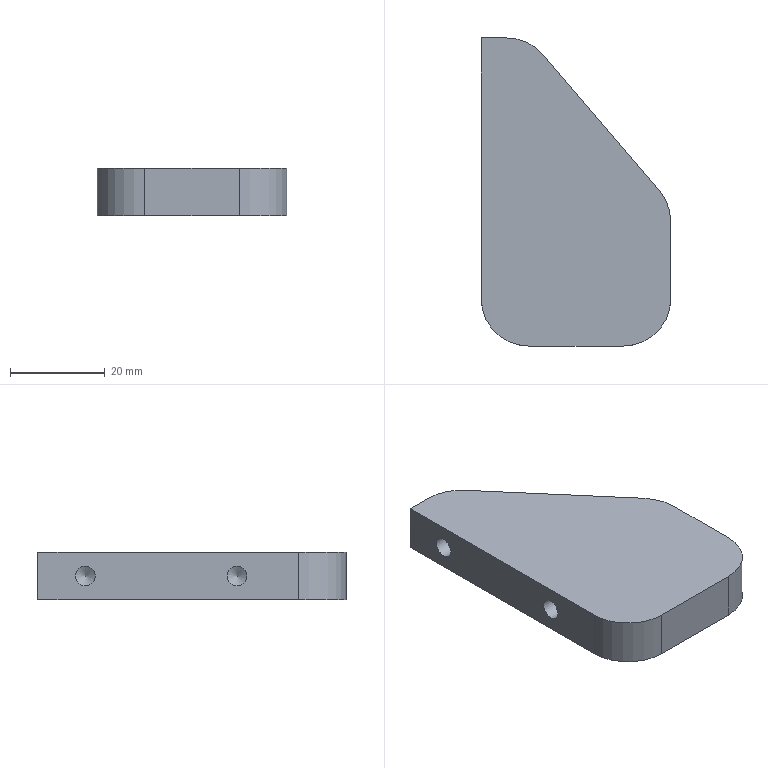Part | NX | 1 solid | 15 faces | box 40 x 65 x 10 mm | volume 19921 mm3 | plane 7 | cylinder 6 | cone 2 | commonest cylinder face diameters 20 x4 4.2 x2
STEP:
#1=CARTESIAN_POINT('',(-20.,22.5,2.1));
#2=VERTEX_POINT('',#1);
#3=CARTESIAN_POINT('',(-20.,22.5,0.));
#4=DIRECTION('',(-1.,0.,0.));
#5=DIRECTION('',(0.,0.,1.));
#6=AXIS2_PLACEMENT_3D('',#3,#4,#5);
#7=CIRCLE('',#6,2.1);
#8=EDGE_CURVE('',#2,#2,#7,.T.);
#9=ORIENTED_EDGE('',*,*,#8,.F.);
#10=EDGE_LOOP('',(#9));
#11=FACE_BOUND('',#10,.T.);
#12=CARTESIAN_POINT('',(-20.,-9.5,2.1));
#13=VERTEX_POINT('',#12);
#14=CARTESIAN_POINT('',(-20.,-9.5,0.));
#15=DIRECTION('',(-1.,0.,0.));
#16=DIRECTION('',(0.,0.,1.));
#17=AXIS2_PLACEMENT_3D('',#14,#15,#16);
#18=CIRCLE('',#17,2.1);
#19=EDGE_CURVE('',#13,#13,#18,.T.);
#20=ORIENTED_EDGE('',*,*,#19,.F.);
#21=EDGE_LOOP('',(#20));
#22=FACE_BOUND('',#21,.T.);
#23=CARTESIAN_POINT('',(-20.,32.5,-5.));
#24=VERTEX_POINT('',#23);
#25=CARTESIAN_POINT('',(-20.,-22.5,-5.));
#26=VERTEX_POINT('',#25);
#27=CARTESIAN_POINT('',(-20.,32.5,-5.));
#28=DIRECTION('',(0.,-1.,0.));
#29=VECTOR('',#28,1000.);
#30=LINE('',#27,#29);
#31=EDGE_CURVE('',#24,#26,#30,.T.);
#32=ORIENTED_EDGE('',*,*,#31,.T.);
#33=CARTESIAN_POINT('',(-20.,-22.5,5.));
#34=VERTEX_POINT('',#33);
#35=CARTESIAN_POINT('',(-20.,-22.5,5.));
#36=DIRECTION('',(0.,0.,-1.));
#37=VECTOR('',#36,1000.);
#38=LINE('',#35,#37);
#39=EDGE_CURVE('',#26,#34,#38,.F.);
#40=ORIENTED_EDGE('',*,*,#39,.T.);
#41=CARTESIAN_POINT('',(-20.,32.5,5.));
#42=VERTEX_POINT('',#41);
#43=CARTESIAN_POINT('',(-20.,32.5,5.));
#44=DIRECTION('',(0.,-1.,0.));
#45=VECTOR('',#44,1000.);
#46=LINE('',#43,#45);
#47=EDGE_CURVE('',#42,#34,#46,.T.);
#48=ORIENTED_EDGE('',*,*,#47,.F.);
#49=CARTESIAN_POINT('',(-20.,32.5,5.));
#50=DIRECTION('',(0.,0.,-1.));
#51=VECTOR('',#50,1000.);
#52=LINE('',#49,#51);
#53=EDGE_CURVE('',#42,#24,#52,.T.);
#54=ORIENTED_EDGE('',*,*,#53,.T.);
#55=EDGE_LOOP('',(#32,#40,#48,#54));
#56=FACE_BOUND('',#55,.T.);
#57=CARTESIAN_POINT('',(-20.,32.5,5.));
#58=DIRECTION('',(1.,0.,0.));
#59=DIRECTION('',(0.,1.,0.));
#60=AXIS2_PLACEMENT_3D('',#57,#58,#59);
#61=PLANE('',#60);
#62=ADVANCED_FACE('',(#11,#22,#56),#61,.F.);
#63=CARTESIAN_POINT('',(-10.,-32.5,5.));
#64=VERTEX_POINT('',#63);
#65=CARTESIAN_POINT('',(10.,-32.5,5.));
#66=VERTEX_POINT('',#65);
#67=CARTESIAN_POINT('',(20.,-32.5,5.));
#68=DIRECTION('',(1.,0.,0.));
#69=VECTOR('',#68,1000.);
#70=LINE('',#67,#69);
#71=EDGE_CURVE('',#64,#66,#70,.T.);
#72=ORIENTED_EDGE('',*,*,#71,.F.);
#73=CARTESIAN_POINT('',(-10.,-32.5,-5.));
#74=VERTEX_POINT('',#73);
#75=CARTESIAN_POINT('',(-10.,-32.5,5.));
#76=DIRECTION('',(0.,0.,-1.));
#77=VECTOR('',#76,1000.);
#78=LINE('',#75,#77);
#79=EDGE_CURVE('',#64,#74,#78,.T.);
#80=ORIENTED_EDGE('',*,*,#79,.T.);
#81=CARTESIAN_POINT('',(10.,-32.5,-5.));
#82=VERTEX_POINT('',#81);
#83=CARTESIAN_POINT('',(20.,-32.5,-5.));
#84=DIRECTION('',(1.,0.,0.));
#85=VECTOR('',#84,1000.);
#86=LINE('',#83,#85);
#87=EDGE_CURVE('',#74,#82,#86,.T.);
#88=ORIENTED_EDGE('',*,*,#87,.T.);
#89=CARTESIAN_POINT('',(10.,-32.5,5.));
#90=DIRECTION('',(0.,0.,-1.));
#91=VECTOR('',#90,1000.);
#92=LINE('',#89,#91);
#93=EDGE_CURVE('',#82,#66,#92,.F.);
#94=ORIENTED_EDGE('',*,*,#93,.T.);
#95=EDGE_LOOP('',(#72,#80,#88,#94));
#96=FACE_BOUND('',#95,.T.);
#97=CARTESIAN_POINT('',(20.,-32.5,5.));
#98=DIRECTION('',(0.,1.,0.));
#99=DIRECTION('',(0.,0.,1.));
#100=AXIS2_PLACEMENT_3D('',#97,#98,#99);
#101=PLANE('',#100);
#102=ADVANCED_FACE('',(#96),#101,.F.);
#103=CARTESIAN_POINT('',(20.,-22.5,-5.));
#104=VERTEX_POINT('',#103);
#105=CARTESIAN_POINT('',(20.,-6.199,-5.));
#106=VERTEX_POINT('',#105);
#107=CARTESIAN_POINT('',(20.,32.5,-5.));
#108=DIRECTION('',(0.,1.,0.));
#109=VECTOR('',#108,1000.);
#110=LINE('',#107,#109);
#111=EDGE_CURVE('',#104,#106,#110,.T.);
#112=ORIENTED_EDGE('',*,*,#111,.T.);
#113=CARTESIAN_POINT('',(20.,-6.199,5.));
#114=VERTEX_POINT('',#113);
#115=CARTESIAN_POINT('',(20.,-6.199,5.));
#116=DIRECTION('',(0.,0.,-1.));
#117=VECTOR('',#116,1000.);
#118=LINE('',#115,#117);
#119=EDGE_CURVE('',#106,#114,#118,.F.);
#120=ORIENTED_EDGE('',*,*,#119,.T.);
#121=CARTESIAN_POINT('',(20.,-22.5,5.));
#122=VERTEX_POINT('',#121);
#123=CARTESIAN_POINT('',(20.,32.5,5.));
#124=DIRECTION('',(0.,1.,0.));
#125=VECTOR('',#124,1000.);
#126=LINE('',#123,#125);
#127=EDGE_CURVE('',#122,#114,#126,.T.);
#128=ORIENTED_EDGE('',*,*,#127,.F.);
#129=CARTESIAN_POINT('',(20.,-22.5,5.));
#130=DIRECTION('',(0.,0.,-1.));
#131=VECTOR('',#130,1000.);
#132=LINE('',#129,#131);
#133=EDGE_CURVE('',#122,#104,#132,.T.);
#134=ORIENTED_EDGE('',*,*,#133,.T.);
#135=EDGE_LOOP('',(#112,#120,#128,#134));
#136=FACE_BOUND('',#135,.T.);
#137=CARTESIAN_POINT('',(20.,32.5,5.));
#138=DIRECTION('',(-1.,0.,0.));
#139=DIRECTION('',(0.,-1.,0.));
#140=AXIS2_PLACEMENT_3D('',#137,#138,#139);
#141=PLANE('',#140);
#142=ADVANCED_FACE('',(#136),#141,.F.);
#143=CARTESIAN_POINT('',(-14.599,32.5,5.));
#144=VERTEX_POINT('',#143);
#145=CARTESIAN_POINT('',(20.,32.5,5.));
#146=DIRECTION('',(-1.,0.,0.));
#147=VECTOR('',#146,1000.);
#148=LINE('',#145,#147);
#149=EDGE_CURVE('',#144,#42,#148,.T.);
#150=ORIENTED_EDGE('',*,*,#149,.F.);
#151=CARTESIAN_POINT('',(-14.599,32.5,-5.));
#152=VERTEX_POINT('',#151);
#153=CARTESIAN_POINT('',(-14.599,32.5,-5.));
#154=DIRECTION('',(0.,0.,1.));
#155=VECTOR('',#154,1000.);
#156=LINE('',#153,#155);
#157=EDGE_CURVE('',#144,#152,#156,.F.);
#158=ORIENTED_EDGE('',*,*,#157,.T.);
#159=CARTESIAN_POINT('',(20.,32.5,-5.));
#160=DIRECTION('',(-1.,0.,0.));
#161=VECTOR('',#160,1000.);
#162=LINE('',#159,#161);
#163=EDGE_CURVE('',#152,#24,#162,.T.);
#164=ORIENTED_EDGE('',*,*,#163,.T.);
#165=ORIENTED_EDGE('',*,*,#53,.F.);
#166=EDGE_LOOP('',(#150,#158,#164,#165));
#167=FACE_BOUND('',#166,.T.);
#168=CARTESIAN_POINT('',(20.,32.5,5.));
#169=DIRECTION('',(0.,-1.,0.));
#170=DIRECTION('',(1.,0.,0.));
#171=AXIS2_PLACEMENT_3D('',#168,#169,#170);
#172=PLANE('',#171);
#173=ADVANCED_FACE('',(#167),#172,.F.);
#174=ORIENTED_EDGE('',*,*,#127,.T.);
#175=CARTESIAN_POINT('',(17.593,0.3087,5.));
#176=VERTEX_POINT('',#175);
#177=CARTESIAN_POINT('',(10.,-6.199,5.));
#178=DIRECTION('',(0.,0.,-1.));
#179=DIRECTION('',(-1.,0.,0.));
#180=AXIS2_PLACEMENT_3D('',#177,#178,#179);
#181=CIRCLE('',#180,10.);
#182=EDGE_CURVE('',#114,#176,#181,.F.);
#183=ORIENTED_EDGE('',*,*,#182,.T.);
#184=CARTESIAN_POINT('',(-7.007,29.008,5.));
#185=VERTEX_POINT('',#184);
#186=CARTESIAN_POINT('',(-10.,32.5,5.));
#187=DIRECTION('',(0.6508,-0.7593,0.));
#188=VECTOR('',#187,1000.);
#189=LINE('',#186,#188);
#190=EDGE_CURVE('',#176,#185,#189,.F.);
#191=ORIENTED_EDGE('',*,*,#190,.T.);
#192=CARTESIAN_POINT('',(-14.599,22.5,5.));
#193=DIRECTION('',(0.,0.,-1.));
#194=DIRECTION('',(-1.,0.,0.));
#195=AXIS2_PLACEMENT_3D('',#192,#193,#194);
#196=CIRCLE('',#195,10.);
#197=EDGE_CURVE('',#185,#144,#196,.F.);
#198=ORIENTED_EDGE('',*,*,#197,.T.);
#199=ORIENTED_EDGE('',*,*,#149,.T.);
#200=ORIENTED_EDGE('',*,*,#47,.T.);
#201=CARTESIAN_POINT('',(-10.,-22.5,5.));
#202=DIRECTION('',(0.,0.,-1.));
#203=DIRECTION('',(-1.,0.,0.));
#204=AXIS2_PLACEMENT_3D('',#201,#202,#203);
#205=CIRCLE('',#204,10.);
#206=EDGE_CURVE('',#34,#64,#205,.F.);
#207=ORIENTED_EDGE('',*,*,#206,.T.);
#208=ORIENTED_EDGE('',*,*,#71,.T.);
#209=CARTESIAN_POINT('',(10.,-22.5,5.));
#210=DIRECTION('',(0.,0.,-1.));
#211=DIRECTION('',(-1.,0.,0.));
#212=AXIS2_PLACEMENT_3D('',#209,#210,#211);
#213=CIRCLE('',#212,10.);
#214=EDGE_CURVE('',#66,#122,#213,.F.);
#215=ORIENTED_EDGE('',*,*,#214,.T.);
#216=EDGE_LOOP('',(#174,#183,#191,#198,#199,#200,#207,#208,#215));
#217=FACE_BOUND('',#216,.T.);
#218=CARTESIAN_POINT('',(0.,0.,5.));
#219=DIRECTION('',(0.,0.,-1.));
#220=DIRECTION('',(-1.,0.,0.));
#221=AXIS2_PLACEMENT_3D('',#218,#219,#220);
#222=PLANE('',#221);
#223=ADVANCED_FACE('',(#217),#222,.F.);
#224=CARTESIAN_POINT('',(-7.007,29.008,-5.));
#225=VERTEX_POINT('',#224);
#226=CARTESIAN_POINT('',(17.593,0.3087,-5.));
#227=VERTEX_POINT('',#226);
#228=CARTESIAN_POINT('',(10.294,8.824,-5.));
#229=DIRECTION('',(-0.6508,0.7593,0.));
#230=VECTOR('',#229,1000.);
#231=LINE('',#228,#230);
#232=EDGE_CURVE('',#225,#227,#231,.F.);
#233=ORIENTED_EDGE('',*,*,#232,.T.);
#234=CARTESIAN_POINT('',(10.,-6.199,-5.));
#235=DIRECTION('',(0.,0.,-1.));
#236=DIRECTION('',(-1.,0.,0.));
#237=AXIS2_PLACEMENT_3D('',#234,#235,#236);
#238=CIRCLE('',#237,10.);
#239=EDGE_CURVE('',#227,#106,#238,.T.);
#240=ORIENTED_EDGE('',*,*,#239,.T.);
#241=ORIENTED_EDGE('',*,*,#111,.F.);
#242=CARTESIAN_POINT('',(10.,-22.5,-5.));
#243=DIRECTION('',(0.,0.,-1.));
#244=DIRECTION('',(-1.,0.,0.));
#245=AXIS2_PLACEMENT_3D('',#242,#243,#244);
#246=CIRCLE('',#245,10.);
#247=EDGE_CURVE('',#104,#82,#246,.T.);
#248=ORIENTED_EDGE('',*,*,#247,.T.);
#249=ORIENTED_EDGE('',*,*,#87,.F.);
#250=CARTESIAN_POINT('',(-10.,-22.5,-5.));
#251=DIRECTION('',(0.,0.,-1.));
#252=DIRECTION('',(-1.,0.,0.));
#253=AXIS2_PLACEMENT_3D('',#250,#251,#252);
#254=CIRCLE('',#253,10.);
#255=EDGE_CURVE('',#74,#26,#254,.T.);
#256=ORIENTED_EDGE('',*,*,#255,.T.);
#257=ORIENTED_EDGE('',*,*,#31,.F.);
#258=ORIENTED_EDGE('',*,*,#163,.F.);
#259=CARTESIAN_POINT('',(-14.599,22.5,-5.));
#260=DIRECTION('',(0.,0.,-1.));
#261=DIRECTION('',(-1.,0.,0.));
#262=AXIS2_PLACEMENT_3D('',#259,#260,#261);
#263=CIRCLE('',#262,10.);
#264=EDGE_CURVE('',#152,#225,#263,.T.);
#265=ORIENTED_EDGE('',*,*,#264,.T.);
#266=EDGE_LOOP('',(#233,#240,#241,#248,#249,#256,#257,#258,#265));
#267=FACE_BOUND('',#266,.T.);
#268=CARTESIAN_POINT('',(0.,0.,-5.));
#269=DIRECTION('',(0.,0.,-1.));
#270=DIRECTION('',(-1.,0.,0.));
#271=AXIS2_PLACEMENT_3D('',#268,#269,#270);
#272=PLANE('',#271);
#273=ADVANCED_FACE('',(#267),#272,.T.);
#274=ORIENTED_EDGE('',*,*,#190,.F.);
#275=CARTESIAN_POINT('',(17.593,0.3087,-5.));
#276=DIRECTION('',(0.,0.,1.));
#277=VECTOR('',#276,1000.);
#278=LINE('',#275,#277);
#279=EDGE_CURVE('',#176,#227,#278,.F.);
#280=ORIENTED_EDGE('',*,*,#279,.T.);
#281=ORIENTED_EDGE('',*,*,#232,.F.);
#282=CARTESIAN_POINT('',(-7.007,29.008,5.));
#283=DIRECTION('',(0.,0.,-1.));
#284=VECTOR('',#283,1000.);
#285=LINE('',#282,#284);
#286=EDGE_CURVE('',#225,#185,#285,.F.);
#287=ORIENTED_EDGE('',*,*,#286,.T.);
#288=EDGE_LOOP('',(#274,#280,#281,#287));
#289=FACE_BOUND('',#288,.T.);
#290=CARTESIAN_POINT('',(-10.,32.5,5.));
#291=DIRECTION('',(-0.7593,-0.6508,0.));
#292=DIRECTION('',(0.,0.,-1.));
#293=AXIS2_PLACEMENT_3D('',#290,#291,#292);
#294=PLANE('',#293);
#295=ADVANCED_FACE('',(#289),#294,.F.);
#296=CARTESIAN_POINT('',(-6.338,-9.5,0.));
#297=VERTEX_POINT('',#296);
#298=VERTEX_LOOP('',#297);
#299=FACE_BOUND('',#298,.T.);
#300=CARTESIAN_POINT('',(-7.6,-9.5,2.1));
#301=VERTEX_POINT('',#300);
#302=CARTESIAN_POINT('',(-7.6,-9.5,0.));
#303=DIRECTION('',(-1.,0.,0.));
#304=DIRECTION('',(0.,0.,1.));
#305=AXIS2_PLACEMENT_3D('',#302,#303,#304);
#306=CIRCLE('',#305,2.1);
#307=EDGE_CURVE('',#301,#301,#306,.T.);
#308=ORIENTED_EDGE('',*,*,#307,.T.);
#309=EDGE_LOOP('',(#308));
#310=FACE_BOUND('',#309,.T.);
#311=CARTESIAN_POINT('',(-7.6,-9.5,0.));
#312=DIRECTION('',(-1.,0.,0.));
#313=DIRECTION('',(0.,0.,1.));
#314=AXIS2_PLACEMENT_3D('',#311,#312,#313);
#315=CONICAL_SURFACE('',#314,2.1,1.03);
#316=ADVANCED_FACE('',(#299,#310),#315,.F.);
#317=ORIENTED_EDGE('',*,*,#307,.F.);
#318=EDGE_LOOP('',(#317));
#319=FACE_BOUND('',#318,.T.);
#320=ORIENTED_EDGE('',*,*,#19,.T.);
#321=EDGE_LOOP('',(#320));
#322=FACE_BOUND('',#321,.T.);
#323=CARTESIAN_POINT('',(-20.,-9.5,0.));
#324=DIRECTION('',(-1.,0.,0.));
#325=DIRECTION('',(0.,0.,1.));
#326=AXIS2_PLACEMENT_3D('',#323,#324,#325);
#327=CYLINDRICAL_SURFACE('',#326,2.1);
#328=ADVANCED_FACE('',(#319,#322),#327,.F.);
#329=CARTESIAN_POINT('',(-6.338,22.5,0.));
#330=VERTEX_POINT('',#329);
#331=VERTEX_LOOP('',#330);
#332=FACE_BOUND('',#331,.T.);
#333=CARTESIAN_POINT('',(-7.6,22.5,2.1));
#334=VERTEX_POINT('',#333);
#335=CARTESIAN_POINT('',(-7.6,22.5,0.));
#336=DIRECTION('',(-1.,0.,0.));
#337=DIRECTION('',(0.,0.,1.));
#338=AXIS2_PLACEMENT_3D('',#335,#336,#337);
#339=CIRCLE('',#338,2.1);
#340=EDGE_CURVE('',#334,#334,#339,.T.);
#341=ORIENTED_EDGE('',*,*,#340,.T.);
#342=EDGE_LOOP('',(#341));
#343=FACE_BOUND('',#342,.T.);
#344=CARTESIAN_POINT('',(-7.6,22.5,0.));
#345=DIRECTION('',(-1.,0.,0.));
#346=DIRECTION('',(0.,0.,1.));
#347=AXIS2_PLACEMENT_3D('',#344,#345,#346);
#348=CONICAL_SURFACE('',#347,2.1,1.03);
#349=ADVANCED_FACE('',(#332,#343),#348,.F.);
#350=ORIENTED_EDGE('',*,*,#340,.F.);
#351=EDGE_LOOP('',(#350));
#352=FACE_BOUND('',#351,.T.);
#353=ORIENTED_EDGE('',*,*,#8,.T.);
#354=EDGE_LOOP('',(#353));
#355=FACE_BOUND('',#354,.T.);
#356=CARTESIAN_POINT('',(-20.,22.5,0.));
#357=DIRECTION('',(-1.,0.,0.));
#358=DIRECTION('',(0.,0.,1.));
#359=AXIS2_PLACEMENT_3D('',#356,#357,#358);
#360=CYLINDRICAL_SURFACE('',#359,2.1);
#361=ADVANCED_FACE('',(#352,#355),#360,.F.);
#362=ORIENTED_EDGE('',*,*,#239,.F.);
#363=ORIENTED_EDGE('',*,*,#279,.F.);
#364=ORIENTED_EDGE('',*,*,#182,.F.);
#365=ORIENTED_EDGE('',*,*,#119,.F.);
#366=EDGE_LOOP('',(#362,#363,#364,#365));
#367=FACE_BOUND('',#366,.T.);
#368=CARTESIAN_POINT('',(10.,-6.199,5.));
#369=DIRECTION('',(0.,0.,1.));
#370=DIRECTION('',(1.,0.,0.));
#371=AXIS2_PLACEMENT_3D('',#368,#369,#370);
#372=CYLINDRICAL_SURFACE('',#371,10.);
#373=ADVANCED_FACE('',(#367),#372,.T.);
#374=ORIENTED_EDGE('',*,*,#197,.F.);
#375=ORIENTED_EDGE('',*,*,#286,.F.);
#376=ORIENTED_EDGE('',*,*,#264,.F.);
#377=ORIENTED_EDGE('',*,*,#157,.F.);
#378=EDGE_LOOP('',(#374,#375,#376,#377));
#379=FACE_BOUND('',#378,.T.);
#380=CARTESIAN_POINT('',(-14.599,22.5,5.));
#381=DIRECTION('',(0.,0.,-1.));
#382=DIRECTION('',(-1.,0.,0.));
#383=AXIS2_PLACEMENT_3D('',#380,#381,#382);
#384=CYLINDRICAL_SURFACE('',#383,10.);
#385=ADVANCED_FACE('',(#379),#384,.T.);
#386=ORIENTED_EDGE('',*,*,#206,.F.);
#387=ORIENTED_EDGE('',*,*,#39,.F.);
#388=ORIENTED_EDGE('',*,*,#255,.F.);
#389=ORIENTED_EDGE('',*,*,#79,.F.);
#390=EDGE_LOOP('',(#386,#387,#388,#389));
#391=FACE_BOUND('',#390,.T.);
#392=CARTESIAN_POINT('',(-10.,-22.5,5.));
#393=DIRECTION('',(0.,0.,-1.));
#394=DIRECTION('',(-1.,0.,0.));
#395=AXIS2_PLACEMENT_3D('',#392,#393,#394);
#396=CYLINDRICAL_SURFACE('',#395,10.);
#397=ADVANCED_FACE('',(#391),#396,.T.);
#398=ORIENTED_EDGE('',*,*,#214,.F.);
#399=ORIENTED_EDGE('',*,*,#93,.F.);
#400=ORIENTED_EDGE('',*,*,#247,.F.);
#401=ORIENTED_EDGE('',*,*,#133,.F.);
#402=EDGE_LOOP('',(#398,#399,#400,#401));
#403=FACE_BOUND('',#402,.T.);
#404=CARTESIAN_POINT('',(10.,-22.5,5.));
#405=DIRECTION('',(0.,0.,-1.));
#406=DIRECTION('',(-1.,0.,0.));
#407=AXIS2_PLACEMENT_3D('',#404,#405,#406);
#408=CYLINDRICAL_SURFACE('',#407,10.);
#409=ADVANCED_FACE('',(#403),#408,.T.);
#410=CLOSED_SHELL('',(#62,#102,#142,#173,#223,#273,#295,#316,#328,#349,#361,#373,#385,#397,#409));
#411=MANIFOLD_SOLID_BREP('',#410);
#412=(LENGTH_UNIT()NAMED_UNIT(*)SI_UNIT(.MILLI.,.METRE.));
#413=UNCERTAINTY_MEASURE_WITH_UNIT(LENGTH_MEASURE(0.00001),#412,'','');
#414=(NAMED_UNIT(*)PLANE_ANGLE_UNIT()SI_UNIT($,.RADIAN.));
#415=(NAMED_UNIT(*)SI_UNIT($,.STERADIAN.)SOLID_ANGLE_UNIT());
#416=(GEOMETRIC_REPRESENTATION_CONTEXT(3)GLOBAL_UNCERTAINTY_ASSIGNED_CONTEXT((#413))GLOBAL_UNIT_ASSIGNED_CONTEXT((#412,#414,#415))REPRESENTATION_CONTEXT('',''));
#417=ADVANCED_BREP_SHAPE_REPRESENTATION('',(#411),#416);